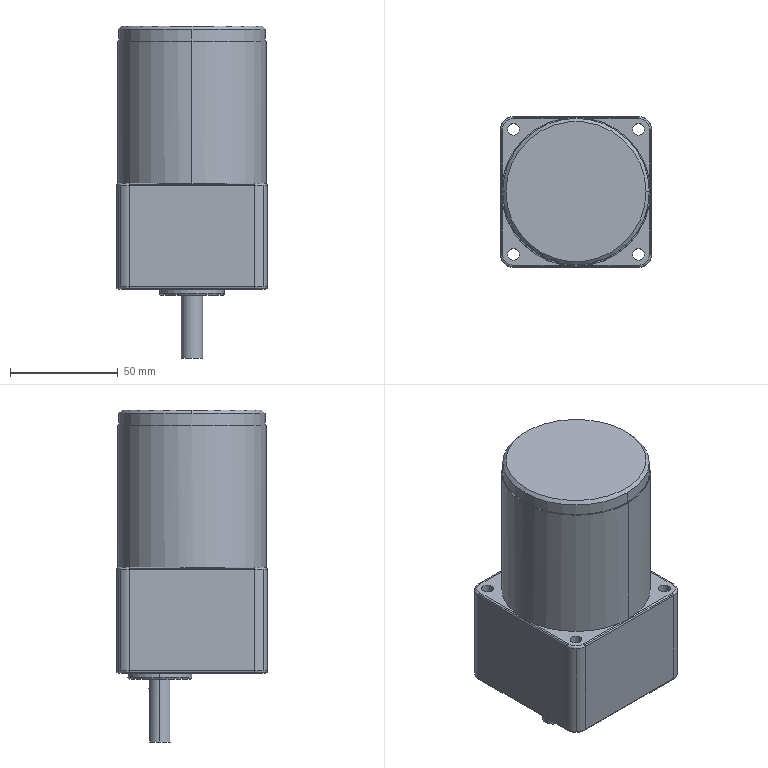Part | NX | 1 solid | 72 faces | box 70 x 70 x 154 mm | volume 504917 mm3 | cylinder 43 | plane 17 | torus 10 | cone 2 | commonest cylinder face diameters 2 x16 5.5 x8 12 x8 10 x2 30 x2 64 x2